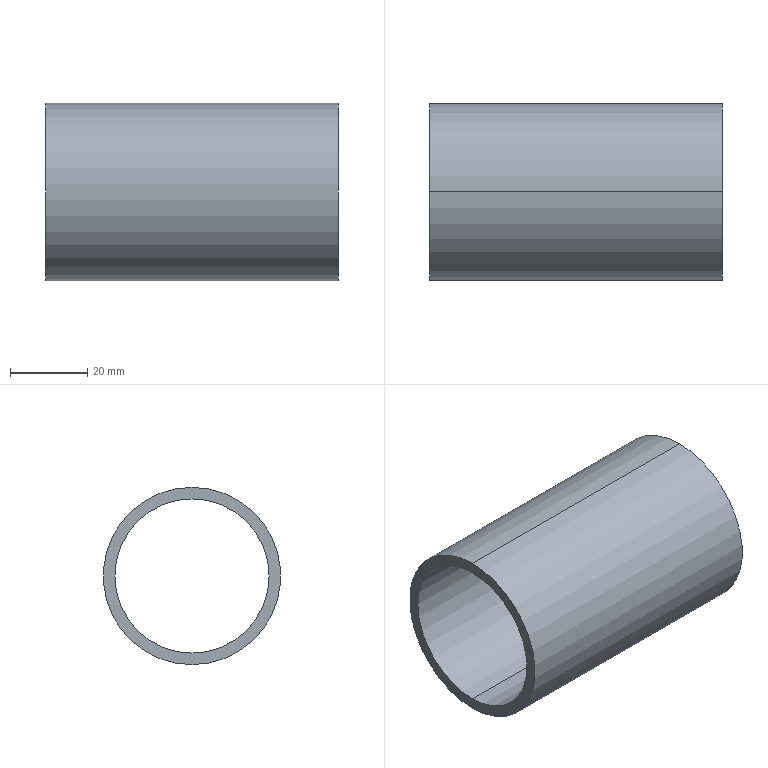Part | SolidWorks | features Extrusion 1 | 1 solid | 6 faces | box 76 x 46 x 46 mm | volume 30800 mm3 | cylinder 4 | plane 2 | commonest cylinder face diameters 40 x2 46 x2
STEP:
#1=CARTESIAN_POINT('',(76.,0.,20.));
#2=VERTEX_POINT('',#1);
#3=CARTESIAN_POINT('',(76.,0.,-20.));
#4=VERTEX_POINT('',#3);
#5=CARTESIAN_POINT('',(76.,0.,0.));
#6=DIRECTION('',(1.,0.,0.));
#7=DIRECTION('',(0.,0.,-1.));
#8=AXIS2_PLACEMENT_3D('',#5,#6,#7);
#9=CIRCLE('',#8,20.);
#10=EDGE_CURVE('',#2,#4,#9,.T.);
#11=ORIENTED_EDGE('',*,*,#10,.T.);
#12=CARTESIAN_POINT('',(0.,0.,-20.));
#13=VERTEX_POINT('',#12);
#14=CARTESIAN_POINT('',(76.,0.,-20.));
#15=DIRECTION('',(-1.,0.,0.));
#16=VECTOR('',#15,1000.);
#17=LINE('',#14,#16);
#18=EDGE_CURVE('',#4,#13,#17,.T.);
#19=ORIENTED_EDGE('',*,*,#18,.T.);
#20=CARTESIAN_POINT('',(0.,0.,20.));
#21=VERTEX_POINT('',#20);
#22=CARTESIAN_POINT('',(0.,0.,0.));
#23=DIRECTION('',(1.,0.,0.));
#24=DIRECTION('',(0.,0.,-1.));
#25=AXIS2_PLACEMENT_3D('',#22,#23,#24);
#26=CIRCLE('',#25,20.);
#27=EDGE_CURVE('',#21,#13,#26,.T.);
#28=ORIENTED_EDGE('',*,*,#27,.F.);
#29=CARTESIAN_POINT('',(76.,0.,20.));
#30=DIRECTION('',(-1.,0.,0.));
#31=VECTOR('',#30,1000.);
#32=LINE('',#29,#31);
#33=EDGE_CURVE('',#2,#21,#32,.T.);
#34=ORIENTED_EDGE('',*,*,#33,.F.);
#35=EDGE_LOOP('',(#11,#19,#28,#34));
#36=FACE_OUTER_BOUND('',#35,.T.);
#37=CARTESIAN_POINT('',(76.,0.,0.));
#38=DIRECTION('',(-1.,0.,0.));
#39=DIRECTION('',(0.,0.,1.));
#40=AXIS2_PLACEMENT_3D('',#37,#38,#39);
#41=CYLINDRICAL_SURFACE('',#40,20.);
#42=ADVANCED_FACE('',(#36),#41,.F.);
#43=CARTESIAN_POINT('',(76.,0.,-23.));
#44=VERTEX_POINT('',#43);
#45=CARTESIAN_POINT('',(76.,0.,23.));
#46=VERTEX_POINT('',#45);
#47=CARTESIAN_POINT('',(76.,0.,0.));
#48=DIRECTION('',(1.,0.,0.));
#49=DIRECTION('',(0.,0.,-1.));
#50=AXIS2_PLACEMENT_3D('',#47,#48,#49);
#51=CIRCLE('',#50,23.);
#52=EDGE_CURVE('',#44,#46,#51,.T.);
#53=ORIENTED_EDGE('',*,*,#52,.F.);
#54=CARTESIAN_POINT('',(0.,0.,-23.));
#55=VERTEX_POINT('',#54);
#56=CARTESIAN_POINT('',(76.,0.,-23.));
#57=DIRECTION('',(-1.,0.,0.));
#58=VECTOR('',#57,1000.);
#59=LINE('',#56,#58);
#60=EDGE_CURVE('',#44,#55,#59,.T.);
#61=ORIENTED_EDGE('',*,*,#60,.T.);
#62=CARTESIAN_POINT('',(0.,0.,23.));
#63=VERTEX_POINT('',#62);
#64=CARTESIAN_POINT('',(0.,0.,0.));
#65=DIRECTION('',(1.,0.,0.));
#66=DIRECTION('',(0.,0.,-1.));
#67=AXIS2_PLACEMENT_3D('',#64,#65,#66);
#68=CIRCLE('',#67,23.);
#69=EDGE_CURVE('',#55,#63,#68,.T.);
#70=ORIENTED_EDGE('',*,*,#69,.T.);
#71=CARTESIAN_POINT('',(76.,0.,23.));
#72=DIRECTION('',(-1.,0.,0.));
#73=VECTOR('',#72,1000.);
#74=LINE('',#71,#73);
#75=EDGE_CURVE('',#46,#63,#74,.T.);
#76=ORIENTED_EDGE('',*,*,#75,.F.);
#77=EDGE_LOOP('',(#53,#61,#70,#76));
#78=FACE_OUTER_BOUND('',#77,.T.);
#79=CARTESIAN_POINT('',(76.,0.,0.));
#80=DIRECTION('',(-1.,0.,0.));
#81=DIRECTION('',(0.,0.,1.));
#82=AXIS2_PLACEMENT_3D('',#79,#80,#81);
#83=CYLINDRICAL_SURFACE('',#82,23.);
#84=ADVANCED_FACE('',(#78),#83,.T.);
#85=CARTESIAN_POINT('',(76.,0.,0.));
#86=DIRECTION('',(1.,0.,0.));
#87=DIRECTION('',(0.,0.,-1.));
#88=AXIS2_PLACEMENT_3D('',#85,#86,#87);
#89=CIRCLE('',#88,23.);
#90=EDGE_CURVE('',#46,#44,#89,.T.);
#91=ORIENTED_EDGE('',*,*,#90,.T.);
#92=ORIENTED_EDGE('',*,*,#52,.T.);
#93=EDGE_LOOP('',(#91,#92));
#94=FACE_OUTER_BOUND('',#93,.T.);
#95=ORIENTED_EDGE('',*,*,#10,.F.);
#96=CARTESIAN_POINT('',(76.,0.,0.));
#97=DIRECTION('',(1.,0.,0.));
#98=DIRECTION('',(0.,0.,-1.));
#99=AXIS2_PLACEMENT_3D('',#96,#97,#98);
#100=CIRCLE('',#99,20.);
#101=EDGE_CURVE('',#4,#2,#100,.T.);
#102=ORIENTED_EDGE('',*,*,#101,.F.);
#103=EDGE_LOOP('',(#95,#102));
#104=FACE_BOUND('',#103,.T.);
#105=CARTESIAN_POINT('',(76.,0.,0.));
#106=DIRECTION('',(1.,0.,0.));
#107=DIRECTION('',(0.,0.,-1.));
#108=AXIS2_PLACEMENT_3D('',#105,#106,#107);
#109=PLANE('',#108);
#110=ADVANCED_FACE('',(#94,#104),#109,.T.);
#111=CARTESIAN_POINT('',(0.,0.,0.));
#112=DIRECTION('',(1.,0.,0.));
#113=DIRECTION('',(0.,0.,-1.));
#114=AXIS2_PLACEMENT_3D('',#111,#112,#113);
#115=CIRCLE('',#114,23.);
#116=EDGE_CURVE('',#63,#55,#115,.T.);
#117=ORIENTED_EDGE('',*,*,#116,.F.);
#118=ORIENTED_EDGE('',*,*,#69,.F.);
#119=EDGE_LOOP('',(#117,#118));
#120=FACE_OUTER_BOUND('',#119,.T.);
#121=ORIENTED_EDGE('',*,*,#27,.T.);
#122=CARTESIAN_POINT('',(0.,0.,0.));
#123=DIRECTION('',(1.,0.,0.));
#124=DIRECTION('',(0.,0.,-1.));
#125=AXIS2_PLACEMENT_3D('',#122,#123,#124);
#126=CIRCLE('',#125,20.);
#127=EDGE_CURVE('',#13,#21,#126,.T.);
#128=ORIENTED_EDGE('',*,*,#127,.T.);
#129=EDGE_LOOP('',(#121,#128));
#130=FACE_BOUND('',#129,.T.);
#131=CARTESIAN_POINT('',(0.,0.,0.));
#132=DIRECTION('',(1.,0.,0.));
#133=DIRECTION('',(0.,0.,-1.));
#134=AXIS2_PLACEMENT_3D('',#131,#132,#133);
#135=PLANE('',#134);
#136=ADVANCED_FACE('',(#120,#130),#135,.F.);
#137=ORIENTED_EDGE('',*,*,#60,.F.);
#138=ORIENTED_EDGE('',*,*,#90,.F.);
#139=ORIENTED_EDGE('',*,*,#75,.T.);
#140=ORIENTED_EDGE('',*,*,#116,.T.);
#141=EDGE_LOOP('',(#137,#138,#139,#140));
#142=FACE_OUTER_BOUND('',#141,.T.);
#143=CARTESIAN_POINT('',(76.,0.,0.));
#144=DIRECTION('',(-1.,0.,0.));
#145=DIRECTION('',(0.,0.,1.));
#146=AXIS2_PLACEMENT_3D('',#143,#144,#145);
#147=CYLINDRICAL_SURFACE('',#146,23.);
#148=ADVANCED_FACE('',(#142),#147,.T.);
#149=ORIENTED_EDGE('',*,*,#18,.F.);
#150=ORIENTED_EDGE('',*,*,#101,.T.);
#151=ORIENTED_EDGE('',*,*,#33,.T.);
#152=ORIENTED_EDGE('',*,*,#127,.F.);
#153=EDGE_LOOP('',(#149,#150,#151,#152));
#154=FACE_OUTER_BOUND('',#153,.T.);
#155=CARTESIAN_POINT('',(76.,0.,0.));
#156=DIRECTION('',(-1.,0.,0.));
#157=DIRECTION('',(0.,0.,1.));
#158=AXIS2_PLACEMENT_3D('',#155,#156,#157);
#159=CYLINDRICAL_SURFACE('',#158,20.);
#160=ADVANCED_FACE('',(#154),#159,.F.);
#161=CLOSED_SHELL('',(#42,#84,#110,#136,#148,#160));
#162=MANIFOLD_SOLID_BREP('',#161);
#163=CARTESIAN_POINT('',(0.,0.,0.));
#164=DIRECTION('',(0.,0.,1.));
#165=DIRECTION('',(1.,0.,0.));
#166=AXIS2_PLACEMENT_3D('',#163,#164,#165);
#167=(LENGTH_UNIT()NAMED_UNIT(*)SI_UNIT(.MILLI.,.METRE.));
#168=UNCERTAINTY_MEASURE_WITH_UNIT(LENGTH_MEASURE(0.00001),#167,'','');
#169=(NAMED_UNIT(*)PLANE_ANGLE_UNIT()SI_UNIT($,.RADIAN.));
#170=(NAMED_UNIT(*)SI_UNIT($,.STERADIAN.)SOLID_ANGLE_UNIT());
#171=(GEOMETRIC_REPRESENTATION_CONTEXT(3)GLOBAL_UNCERTAINTY_ASSIGNED_CONTEXT((#168))GLOBAL_UNIT_ASSIGNED_CONTEXT((#167,#169,#170))REPRESENTATION_CONTEXT('',''));
#172=ADVANCED_BREP_SHAPE_REPRESENTATION('',(#162,#166),#171);